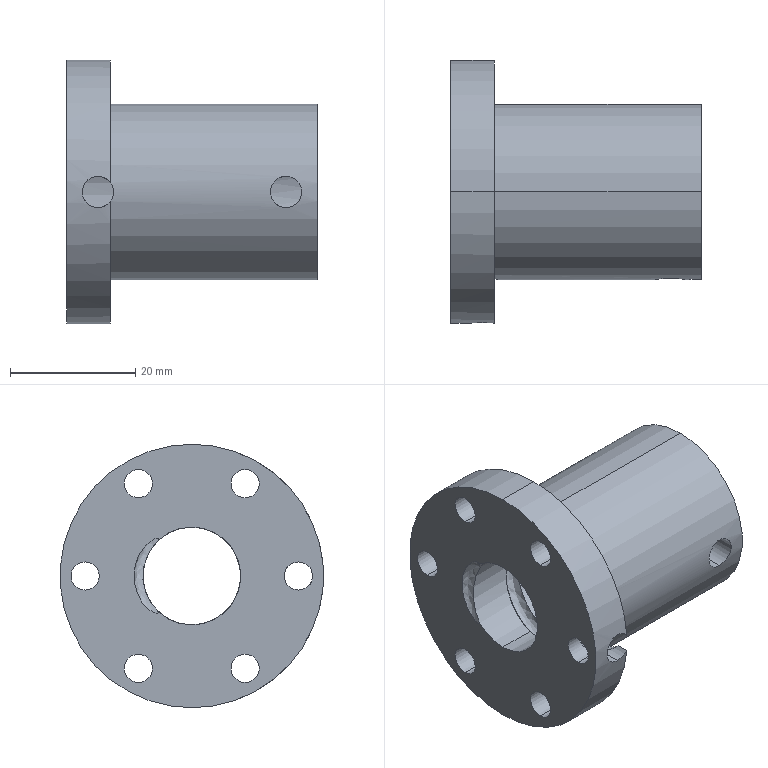Part | SolidWorks | features BaseBody 1 | 1 solid | 50 faces | box 40 x 42 x 42 mm | volume 20795 mm3 | cylinder 39 | spline 6 | plane 5 | commonest cylinder face diameters 4.5 x12 5 x12 15.6 x11 28 x2 42 x2